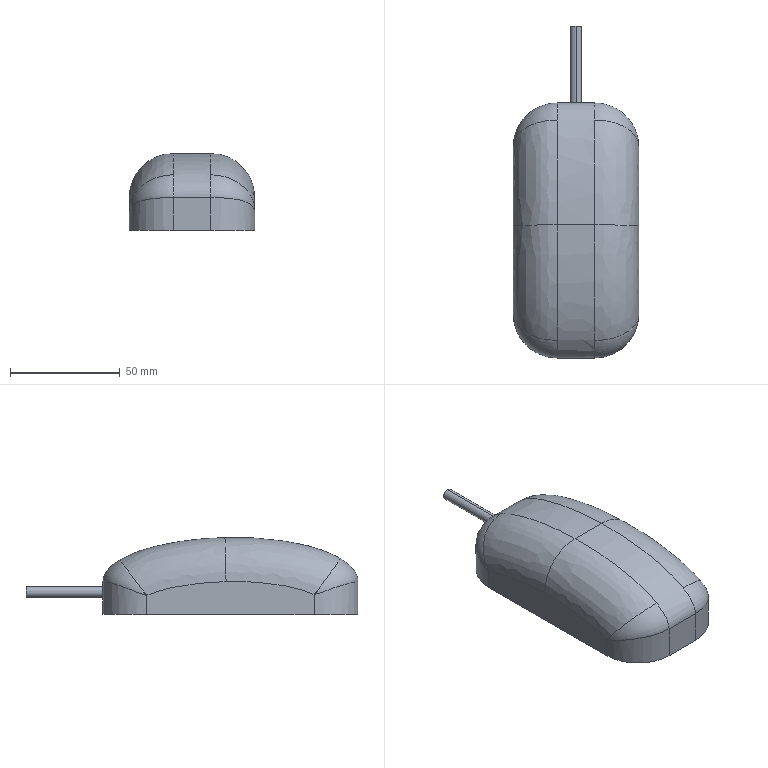Part | STEP file | Shuangfeiyanmouse-OP-520NU2r | 1 solid | 22 faces | box 57 x 151 x 34.996 mm | volume 178729 mm3 | spline 10 | cylinder 6 | plane 6 | commonest cylinder face diameters 40 x4 4.977 x2